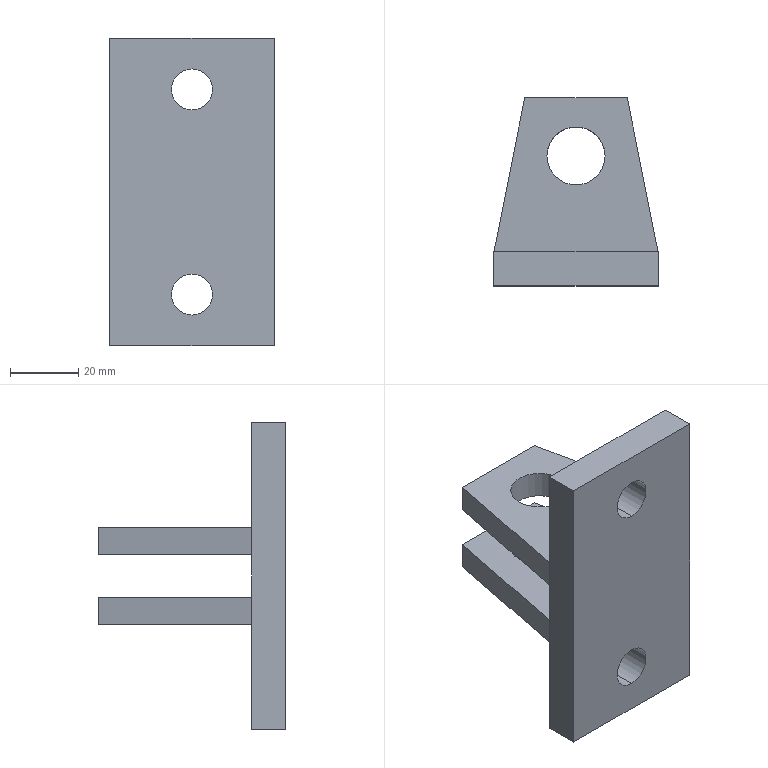Part | STEP file | BCC3 H12_5 | 1 solid | 26 faces | box 48 x 55 x 90 mm | volume 65386 mm3 | plane 18 | cylinder 8 | commonest cylinder face diameters 12 x4 17 x4